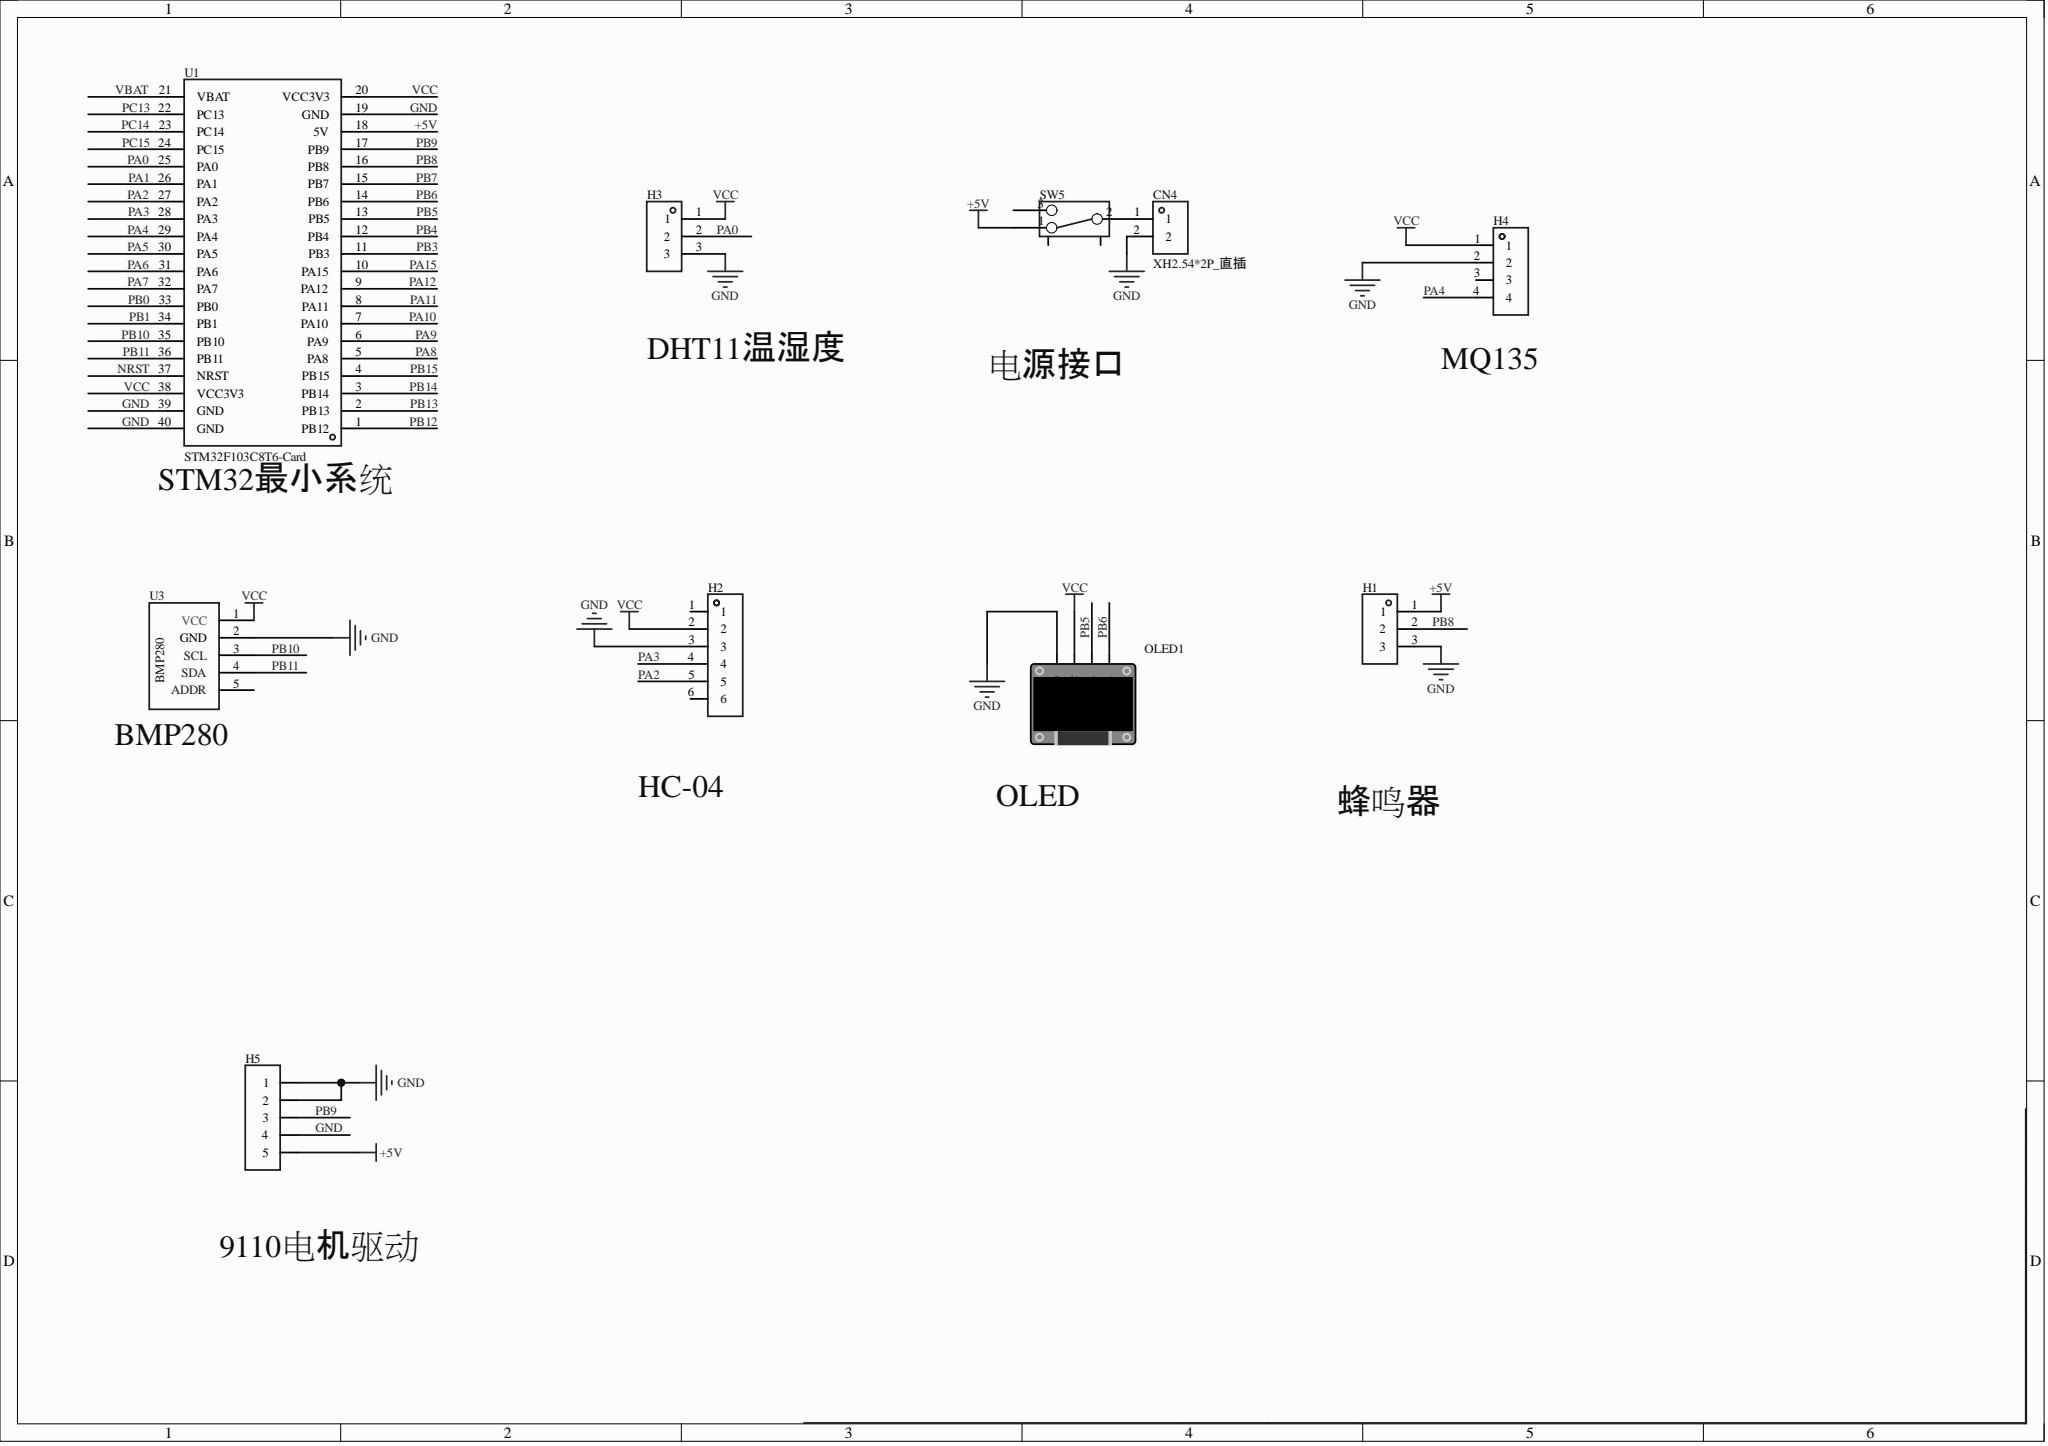Circuit board | Altium Designer | 10 parts | 14 nets
Bill of materials:
Comment,Description,Designator,Footprint,LibRef,Quantity
"XH2.54*2P_直插","","CN4","CONN-TH_2P-P2.50-XH2.54-2P","XH2.54*2P_直插","1"
"","","H1, H3","HDR-TH_3P-P2.54-V-F","HDR-F_2.54_1x3P","2"
"","","H2","HDR-TH_6P-P2.54-V-F","HDR-F_2.54_1x6P","1"
"","","H4","HDR-TH_4P-P2.54-V-F","HDR-F_2.54_1x4P","1"
"","","H5","HDR-TH_5P-P2.54-V-F","HDR-F_2.54_1x5P","1"
"","","OLED1","0.96OLED_4P","0.96OLED模块_4P","1"
"","","SW5","拨动开关","拨动开关_正","1"
"STM32F103C8T6-Card","","U1","CONN-TH_L53.3-W22.9_STM32F103C8T6-CARD","STM32F103C8T6-Card","1"
"","","U3","BH1750光照传感器","BH1750光照传感器","1"
Netlist (Protel format):
[
CN4
CONN-TH_2P-P2.50-XH2.54-2P
XH2.54*2P_直插



]
[
H1
HDR-TH_3P-P2.54-V-F




]
[
H2
HDR-TH_6P-P2.54-V-F




]
[
H3
HDR-TH_3P-P2.54-V-F




]
[
H4
HDR-TH_4P-P2.54-V-F




]
[
H5
HDR-TH_5P-P2.54-V-F




]
[
OLED1
0.96OLED_4P




]
[
SW5
拨动开关




]
[
U1
CONN-TH_L53.3-W22.9_STM32F103C8T6-CARD
STM32F103C8T6-Card



]
[
U3
BH1750光照传感器




]
(
VCC
H2-2
H3-1
H4-1
OLED1-2
U1-20
U1-38
U3-1
)
(
PB11
U1-36
U3-4
)
(
PB10
U1-35
U3-3
)
(
PB9
H5-3
U1-17
)
(
PB8
H1-2
U1-16
)
(
PB6
OLED1-4
U1-14
)
(
PB5
OLED1-3
U1-13
)
(
PA4
H4-4
U1-29
)
(
PA3
H2-4
U1-28
)
(
PA2
H2-5
U1-27
)
(
PA0
H3-2
U1-25
)
(
NetCN4_1
CN4-1
SW5-2
)
(
GND
CN4-2
H1-3
H2-3
H3-3
H4-2
H5-1
H5-2
H5-4
OLED1-1
U1-19
U1-39
U1-40
U3-2
)
(
+5V
H1-1
H5-5
SW5-1
U1-18
)